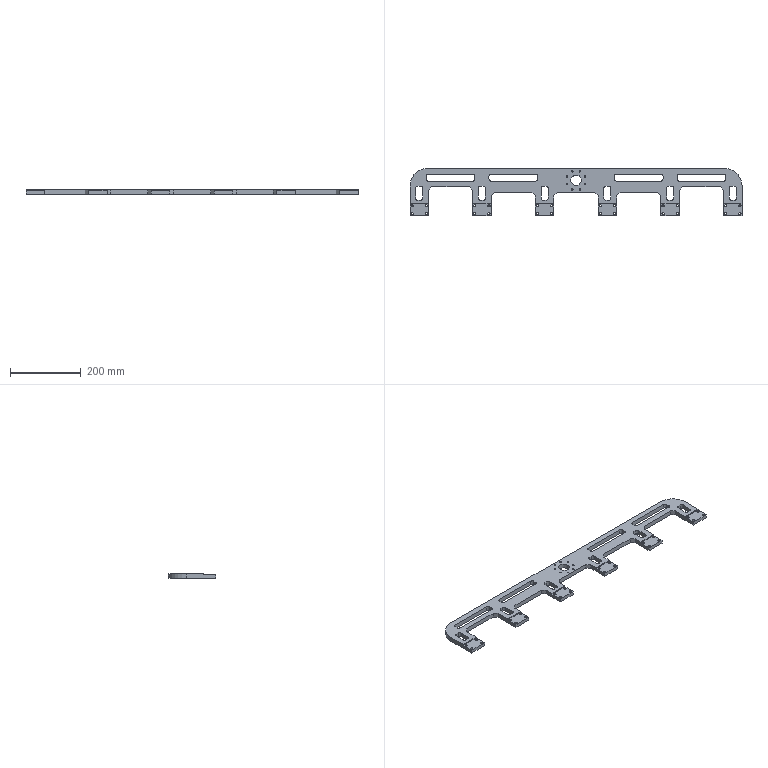NC program | NX | posted with a generic post | part box 941 x 134 x 13 mm
Lines 1 to 99 of 8798:
N10 G17 G21 G94 G90
(FLOOR_WALL_COPY , TOOL : D63)
N12 T01 M6
N14 G54
N16 G17 G0 G90 X-507. Y68.997 S6500 M3
N18 G43 Z30. H1
N20 Z3.
N22 G94 G1 Z0. F1500.
N24 X-504.
N26 X63.089
N28 Y40.798
N30 X-504.
N32 Y12.599
N34 X63.089
N36 Y-15.601
N38 X-504.
N40 Y-43.8
N42 X63.089
N44 Y-71.999
N46 X-504.
N48 X-507.
N50 Z3.
N52 G0 Z30.
N54 M5
(DRILLING_COPY_1 , TOOL : D6A45)
N56 T07 M6
N58 G54
N60 G17 G0 G90 X-464.5 Y-39.2 S5000 M3
N62 G43 Z30. H7
N64 G94 G81 G98 Z-1. F250. R3.
N66 Y-61.2
N68 X-424.5
N70 Y-39.2
N72 X-286.7
N74 Y-61.2
N76 X-246.7
N78 Y-39.2
N80 X-108.9
N82 Y-61.2
N84 X-68.9
N86 Y-39.2
N88 X-10.615 Y7.131
N90 X10.815
N92 X25.969 Y22.285
N94 Y43.715
N96 X10.815 Y58.869
N98 X-10.615
N100 X-25.769 Y43.715
N102 Y22.285
N104 X0.1 Y33.
N106 G80
N108 G0 X0.1 Y33. Z30.
N110 M5
(DRILLING_COPY_COPY_1 , TOOL : 4.5ZT)
N112 T14 M6
N114 G54
N116 G17 G0 G90 X-25.769 Y43.715 S2000 M3
N118 G43 Z30. H14
N120 G94 G83 G98 Z-15.352 F250. Q2. R3.
N122 X-10.615 Y58.869
N124 X10.815
N126 X25.969 Y43.715
N128 Y22.285
N130 X10.815 Y7.131
N132 X-10.615
N134 X-25.769 Y22.285
N136 G80
N138 G0 X-25.769 Y22.285 Z30.
N140 M5
(DRILLING_COPY_COPY_COPY , TOOL : 6.5ZT)
N142 T15 M6
N144 G54
N146 G17 G0 G90 X-464.5 Y-39.2 S2000 M3
N148 G43 Z30. H15
N150 G94 G83 G98 Z-15.953 F250. Q2. R3.
N152 Y-61.2
N154 X-424.5
N156 Y-39.2
N158 X-286.7 Y-61.2
N160 Y-39.2
N162 X-246.7
N164 Y-61.2
N166 X-108.9
N168 Y-39.2
N170 X-68.9
N172 Y-61.2
N174 G80
N176 G0 X-68.9 Y-61.2 Z30.
N178 M5